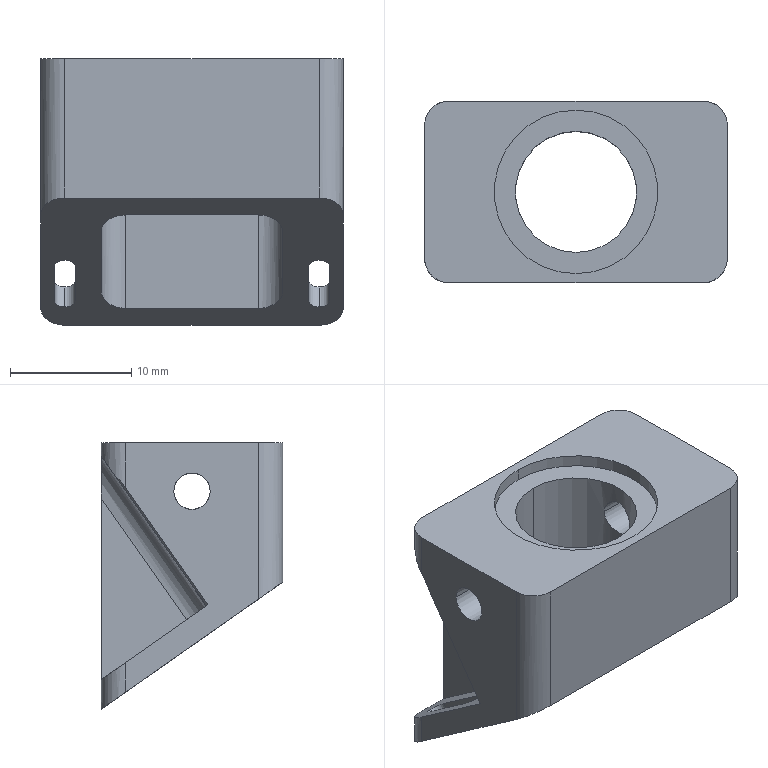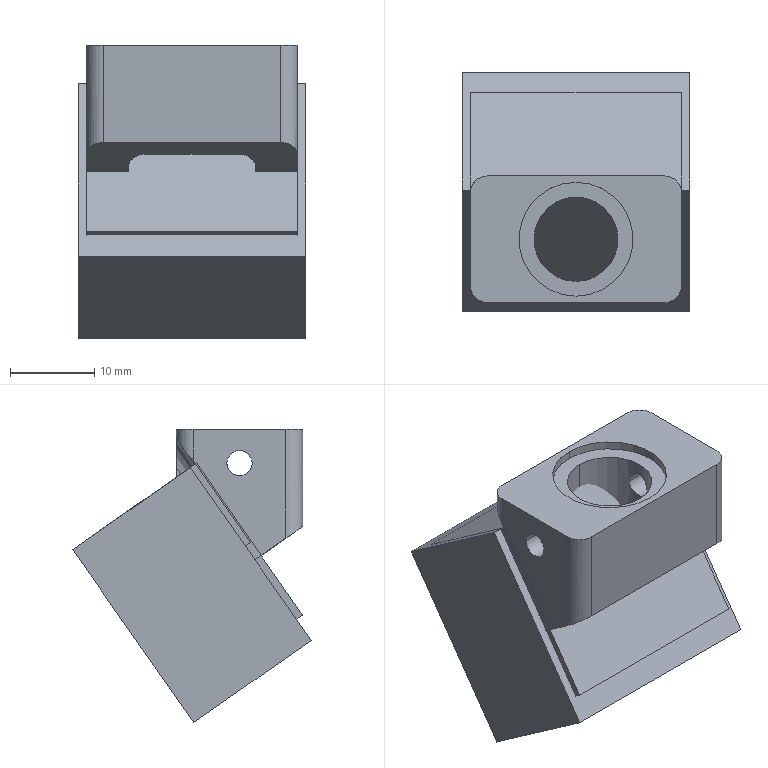CAM job | NX | 3+2 milling, drilling | part box 25 x 15 x 22 mm | stock box 27 x 28.265 x 34.751 mm
Tools:
number,name,description,diameter,corner_radius,flute_length,length,flutes
1,D40面刀,,40.0,0.0,50.0,75.0,2
4,D4点钻,,4.0,0.0,50.0,75.0,2
5,9.5钻头,,9.8,0.0,35.0,50.0,2
2,D8开粗,,8.0,0.0,50.0,75.0,2
3,D8精光,,8.0,0.0,50.0,75.0,2
13,R1,,2.0,1.0,30.0,30.0,4
8,D4开粗,,4.0,0.0,50.0,75.0,2
6,D4精刀,,4.0,0.0,50.0,75.0,2
7,D1精刀,,1.0,0.0,50.0,75.0,2
11,D2.6钻头,,2.6,0.0,35.0,50.0,2
12,丝锥M3,,3.0,0.0,35.0,50.0,4
13,D3点孔,,3.0,0.0,50.0,75.0,2
9,D1.45钻头,,1.45,0.0,35.0,50.0,2
10,丝锥M1.6,,1.6,0.0,35.0,50.0,4
Operations:
program,operation,operation_type,tool,method,geometry_group,spindle_rpm,surface_speed,feed_per_tooth,feed_cut,feed_plunge,cut_length_mm,path_length_mm,cut_time_min,machine_time_min
A1,FACE_MILLING,FaceMilling,D40面刀,MILL_ROUGH,WORKPIECE,3500.0,439.0,0.1143,800.0,60.0,75.0,109.0,0.0979,0.1013
A1,SPOT_DRILLING,Operation,D4点钻,DRILL_METHOD,WORKPIECE,2000.0,25.0,0.0625,250.0,0.0,4.0,48.0,0.016,0.0204
A1,SPOT_DRILLING_COPY,Operation,9.5钻头,DRILL_METHOD,WORKPIECE,1600.0,49.0,0.0781,250.0,0.0,27.0,94.0,0.108,0.1147
A1,PLANAR_MILL,PlanarMilling,D8开粗,MILL_ROUGH,WORKPIECE,4500.0,113.0,0.1667,1500.0,60.0,243.088,323.688,0.1674,0.1755
A1,PLANAR_MILL_COPY_2,PlanarMilling,D8开粗,MILL_ROUGH,WORKPIECE,4500.0,113.0,0.1111,1000.0,60.0,23.326,65.126,0.0257,0.0298
A1,PLANAR_MILL_COPY_1,PlanarMilling,D8精光,MILL_FINISH,WORKPIECE,4500.0,113.0,0.0889,800.0,60.0,117.063,197.663,0.1525,0.1606
A1,PLANAR_MILL_COPY_1_COPY,PlanarMilling,D8精光,MILL_FINISH,WORKPIECE,3500.0,113.0,0.0889,800.0,60.0,25.448,63.448,0.0352,0.039
A1,PLANAR_MILL_COPY,PlanarMilling,R1,MILL_FINISH,WORKPIECE,4500.0,113.0,0.0556,1000.0,60.0,86.293,125.293,0.0881,0.092
A1,PLANAR_MILL_COPY_COPY,PlanarMilling,R1,MILL_FINISH,WORKPIECE,4500.0,113.0,0.0556,1000.0,60.0,43.14,82.14,0.045,0.0489
A1,PLANAR_MILL_COPY_COPY_COPY,PlanarMilling,R1,MILL_FINISH,WORKPIECE,4500.0,113.0,0.0556,1000.0,60.0,33.08,74.08,0.035,0.0391
B1,ADAPTIVE_MILLING,CavityMilling,D4开粗,MILL_ROUGH,WORKPIECE_1,5500.0,69.0,0.1818,2000.0,60.0,723.723,853.299,0.3639,0.3768
B1,PLANAR_MILL_1_COPY,PlanarMilling,D4精刀,MILL_FINISH,WORKPIECE_1,4500.0,56.0,0.0667,600.0,60.0,84.506,320.584,0.1595,0.1831
B1,PLANAR_MILL_1_COPY_COPY,PlanarMilling,D4精刀,MILL_FINISH,WORKPIECE_1,4500.0,56.0,0.0667,600.0,60.0,79.672,364.44,0.1515,0.1799
B1,PLANAR_MILL_1_COPY_COPY_COPY,PlanarMilling,D4精刀,MILL_FINISH,WORKPIECE_1,4500.0,56.0,0.0667,600.0,60.0,79.672,364.44,0.1515,0.1799
C1,PLANAR_MILL_1,PlanarMilling,D40面刀,METHOD,WORKPIECE_2,3500.0,100.0,0.1178,1500.0,100.0,525.0,1015.771,0.35,0.3991
C1,PLANAR_MILL_1_COPY_1,PlanarMilling,D40面刀,METHOD,WORKPIECE_2,3500.0,439.0,0.1143,800.0,100.0,73.0,107.0,0.0912,0.0946
C1,PLANAR_MILL_2,PlanarMilling,D1精刀,MILL_FINISH,WORKPIECE_2,4500.0,21.0,0.0889,800.0,60.0,221.149,281.734,0.4356,0.4422
C1,PLANAR_MILL_2_COPY,PlanarMilling,D1精刀,MILL_FINISH,WORKPIECE_2,6685.0,21.0,0.0299,400.0,60.0,26.227,100.127,0.0671,0.075
C1,PLANAR_MILL_3_COPY,PlanarMilling,R1,MILL_FINISH,WORKPIECE_2,3500.0,43.0,0.1429,1000.0,60.0,28.998,126.699,0.0308,0.0406
C1,PLANAR_MILL_3_COPY_1,PlanarMilling,R1,MILL_FINISH,WORKPIECE_2,3500.0,43.0,0.1429,1000.0,60.0,89.981,128.181,0.0916,0.0954
D1,SPOT_DRILLING_2,Operation,D4点钻,METHOD,WORKPIECE_3,1600.0,20.0,0.0781,250.0,0.0,3.5,47.0,0.014,0.0183
D1,SPOT_DRILLING_2_COPY,Operation,D2.6钻头,METHOD,WORKPIECE_3,1600.0,20.0,0.0781,250.0,0.0,11.0,62.0,0.044,0.0491
D1,SPOT_DRILLING_2_COPY_COPY,Operation,丝锥M3,METHOD,WORKPIECE_3,400.0,3.0,0.0006,0.5,0.0,10.5,61.0,21.0,21.005
E1,SPOT_DRILLING_2_COPY_1,Operation,D4点钻,METHOD,WORKPIECE_4,1600.0,20.0,0.0781,250.0,0.0,3.5,47.0,0.014,0.0183
E1,SPOT_DRILLING_2_COPY_COPY_1,Operation,D2.6钻头,METHOD,WORKPIECE_4,1600.0,20.0,0.0781,250.0,0.0,11.0,62.0,0.044,0.0491
E1,SPOT_DRILLING_2_COPY_COPY_COPY,Operation,丝锥M3,METHOD,WORKPIECE_4,400.0,3.0,0.0006,0.5,0.0,10.5,61.0,21.0,21.005
F1,ADAPTIVE_MILLING_1,CavityMilling,D4开粗,MILL_ROUGH,WORKPIECE_5,5500.0,69.0,0.0227,1000.0,60.0,432.942,472.792,0.4415,0.4455
F1,SPOT_DRILLING_1,Operation,D3点孔,DRILL_METHOD,WORKPIECE_5,1600.0,20.0,0.0781,250.0,0.0,11.2,110.141,0.0448,0.0547
F1,PLANAR_MILL_4,PlanarMilling,D3点孔,METHOD,WORKPIECE_5,3500.0,43.0,0.1429,1000.0,100.0,27.847,84.447,0.0278,0.0335
F1,SPOT_DRILLING_1_COPY,Operation,D1.45钻头,DRILL_METHOD,WORKPIECE_5,1300.0,5.0,0.0577,150.0,0.0,36.0,159.741,0.24,0.2524
F1,SPOT_DRILLING_1_COPY_COPY,Operation,丝锥M1.6,DRILL_METHOD,WORKPIECE_5,300.0,1.0,0.0003,0.35,0.0,38.0,163.741,108.571,108.584
F1,PLANAR_MILL_6,PlanarMilling,D4精刀,MILL_FINISH,WORKPIECE_5,4500.0,56.0,0.0889,800.0,60.0,64.0,116.0,0.0825,0.0877
F1,PLANAR_MILL_6_COPY,PlanarMilling,D4精刀,MILL_FINISH,WORKPIECE_5,4500.0,56.0,0.0444,400.0,60.0,43.142,95.142,0.1138,0.119
F1,PLANAR_MILL_5,PlanarMilling,D8精光,MILL_FINISH,WORKPIECE_5,4500.0,113.0,0.0444,400.0,60.0,18.766,92.366,0.052,0.0593
F1,SOLID_PROFILE_3D,PlanarMilling,R1,METHOD,WORKPIECE_5,3500.0,100.0,0.1178,800.0,100.0,58.335,91.965,0.0729,0.0763